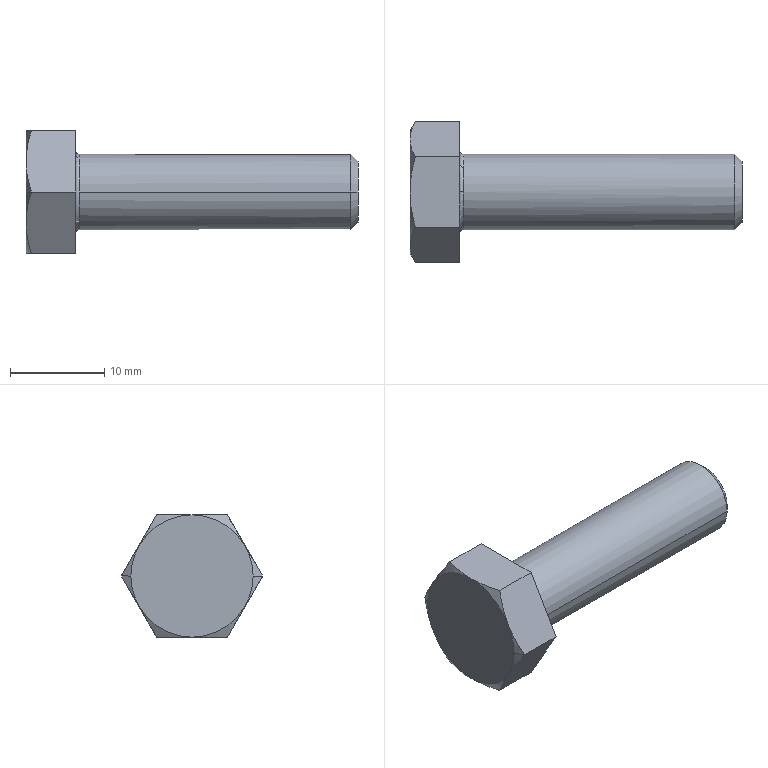Part | STEP file | KS B 1002 - C  M 8 x 30 | 1 solid | 23 faces | box 35.3 x 15.011 x 13 mm | volume 2275 mm3 | cone 10 | plane 9 | torus 2 | cylinder 2 | commonest cylinder face diameters 8 x2